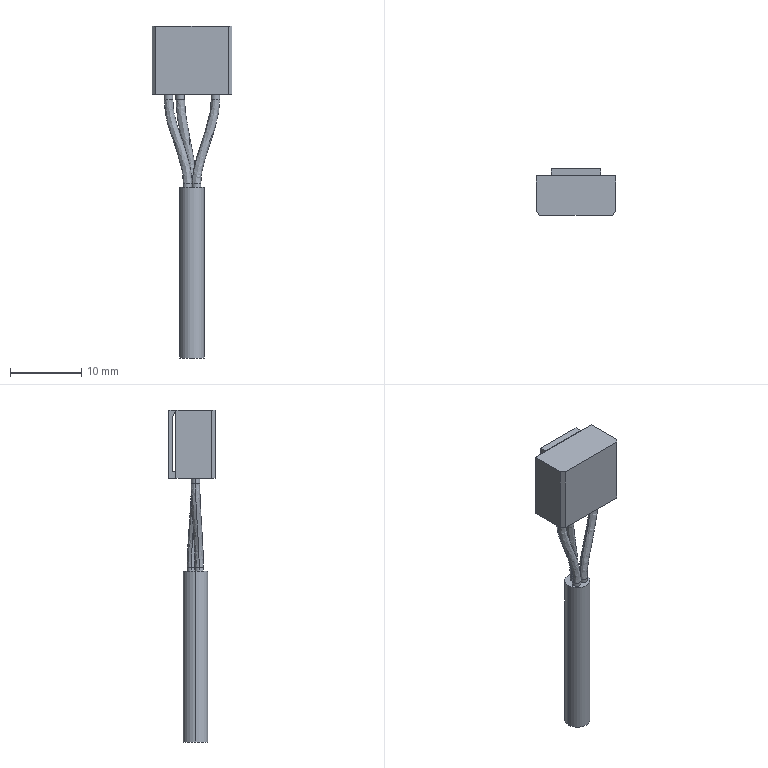Part | SolidWorks | features BaseBody 2 | 2 solids | 40 faces | box 11.2 x 6.5 x 46.6 mm | volume 903.576 mm3 | plane 20 | cylinder 14 | spline 6 | commonest cylinder face diameters 1.2 x12 3.5 x2